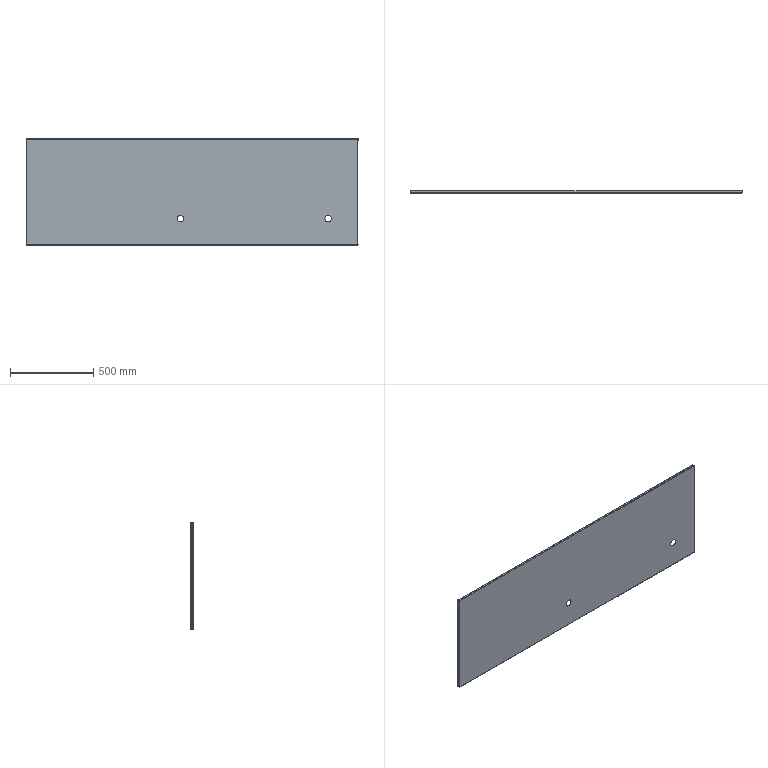Part | STEP file | HESS-408-70-15W-W-16-bottom frame drip tray 1 | 1 solid | 74 faces | box 2000 x 15 x 640 mm | volume 2094402 mm3 | plane 54 | cylinder 20 | commonest cylinder face diameters 0.1 x4 0.2 x4 3.1 x4 3.2 x4 40 x4